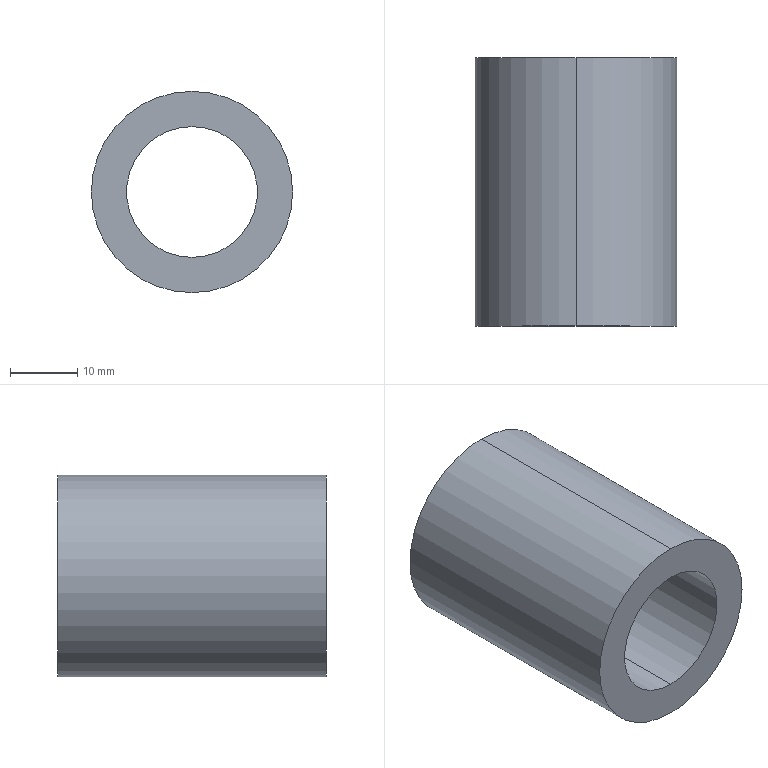Part | STEP file | 1 solid | 6 faces | box 30 x 40 x 30 mm | volume 16328 mm3 | cylinder 4 | plane 2 | commonest cylinder face diameters 19.5 x2 30 x2
STEP:
#1=CARTESIAN_POINT('',(0.,0.,0.));
#2=DIRECTION('',(0.,0.,1.));
#3=DIRECTION('',(1.,0.,0.));
#4=AXIS2_PLACEMENT_3D('',#1,#2,#3);
#5=CARTESIAN_POINT('',(0.,40.,-9.75));
#6=VERTEX_POINT('',#5);
#7=CARTESIAN_POINT('',(0.,0.,-9.75));
#8=VERTEX_POINT('',#7);
#9=CARTESIAN_POINT('',(0.,40.,-9.75));
#10=DIRECTION('',(0.,-1.,0.));
#11=VECTOR('',#10,1.);
#12=LINE('',#9,#11);
#13=CARTESIAN_POINT('',(0.,40.,0.));
#14=DIRECTION('',(0.,-1.,0.));
#15=DIRECTION('',(0.,0.,-1.));
#16=AXIS2_PLACEMENT_3D('',#13,#14,#15);
#17=CYLINDRICAL_SURFACE('',#16,9.75);
#18=CARTESIAN_POINT('',(6.283,0.));
#19=DIRECTION('',(0.,1.));
#20=VECTOR('',#19,1.);
#21=LINE('',#18,#20);
#22=(GEOMETRIC_REPRESENTATION_CONTEXT(2)PARAMETRIC_REPRESENTATION_CONTEXT()REPRESENTATION_CONTEXT('',''));
#23=DEFINITIONAL_REPRESENTATION('',(#21),#22);
#24=PCURVE('',#17,#23);
#25=CARTESIAN_POINT('',(0.,40.,0.));
#26=DIRECTION('',(0.,-1.,0.));
#27=DIRECTION('',(0.,0.,-1.));
#28=AXIS2_PLACEMENT_3D('',#25,#26,#27);
#29=CYLINDRICAL_SURFACE('',#28,9.75);
#30=CARTESIAN_POINT('',(0.,0.));
#31=DIRECTION('',(0.,1.));
#32=VECTOR('',#31,1.);
#33=LINE('',#30,#32);
#34=(GEOMETRIC_REPRESENTATION_CONTEXT(2)PARAMETRIC_REPRESENTATION_CONTEXT()REPRESENTATION_CONTEXT('',''));
#35=DEFINITIONAL_REPRESENTATION('',(#33),#34);
#36=PCURVE('',#29,#35);
#37=SURFACE_CURVE('',#12,(#24,#36),.PCURVE_S1.);
#38=EDGE_CURVE('',#6,#8,#37,.T.);
#39=ORIENTED_EDGE('',*,*,#38,.T.);
#40=CARTESIAN_POINT('',(0.,0.,9.75));
#41=VERTEX_POINT('',#40);
#42=CARTESIAN_POINT('',(0.,0.,0.));
#43=DIRECTION('',(0.,1.,0.));
#44=DIRECTION('',(0.,0.,1.));
#45=AXIS2_PLACEMENT_3D('',#42,#43,#44);
#46=CIRCLE('',#45,9.75);
#47=CARTESIAN_POINT('',(9.425,40.));
#48=DIRECTION('',(-1.,0.));
#49=VECTOR('',#48,1.);
#50=LINE('',#47,#49);
#51=(GEOMETRIC_REPRESENTATION_CONTEXT(2)PARAMETRIC_REPRESENTATION_CONTEXT()REPRESENTATION_CONTEXT('',''));
#52=DEFINITIONAL_REPRESENTATION('',(#50),#51);
#53=PCURVE('',#17,#52);
#54=CARTESIAN_POINT('',(0.,0.,0.));
#55=DIRECTION('',(0.,1.,0.));
#56=DIRECTION('',(0.,0.,1.));
#57=AXIS2_PLACEMENT_3D('',#54,#55,#56);
#58=PLANE('',#57);
#59=CARTESIAN_POINT('',(0.,0.));
#60=DIRECTION('',(1.,0.));
#61=AXIS2_PLACEMENT_2D('',#59,#60);
#62=CIRCLE('',#61,9.75);
#63=(GEOMETRIC_REPRESENTATION_CONTEXT(2)PARAMETRIC_REPRESENTATION_CONTEXT()REPRESENTATION_CONTEXT('',''));
#64=DEFINITIONAL_REPRESENTATION('',(#62),#63);
#65=PCURVE('',#58,#64);
#66=SURFACE_CURVE('',#46,(#53,#65),.PCURVE_S1.);
#67=EDGE_CURVE('',#8,#41,#66,.T.);
#68=ORIENTED_EDGE('',*,*,#67,.T.);
#69=CARTESIAN_POINT('',(0.,40.,9.75));
#70=VERTEX_POINT('',#69);
#71=CARTESIAN_POINT('',(0.,40.,9.75));
#72=DIRECTION('',(0.,-1.,0.));
#73=VECTOR('',#72,1.);
#74=LINE('',#71,#73);
#75=CARTESIAN_POINT('',(3.142,0.));
#76=DIRECTION('',(0.,1.));
#77=VECTOR('',#76,1.);
#78=LINE('',#75,#77);
#79=(GEOMETRIC_REPRESENTATION_CONTEXT(2)PARAMETRIC_REPRESENTATION_CONTEXT()REPRESENTATION_CONTEXT('',''));
#80=DEFINITIONAL_REPRESENTATION('',(#78),#79);
#81=PCURVE('',#17,#80);
#82=CARTESIAN_POINT('',(3.142,0.));
#83=DIRECTION('',(0.,1.));
#84=VECTOR('',#83,1.);
#85=LINE('',#82,#84);
#86=(GEOMETRIC_REPRESENTATION_CONTEXT(2)PARAMETRIC_REPRESENTATION_CONTEXT()REPRESENTATION_CONTEXT('',''));
#87=DEFINITIONAL_REPRESENTATION('',(#85),#86);
#88=PCURVE('',#29,#87);
#89=SURFACE_CURVE('',#74,(#81,#88),.PCURVE_S1.);
#90=EDGE_CURVE('',#70,#41,#89,.T.);
#91=ORIENTED_EDGE('',*,*,#90,.F.);
#92=CARTESIAN_POINT('',(0.,40.,0.));
#93=DIRECTION('',(0.,1.,0.));
#94=DIRECTION('',(0.,0.,1.));
#95=AXIS2_PLACEMENT_3D('',#92,#93,#94);
#96=CIRCLE('',#95,9.75);
#97=CARTESIAN_POINT('',(9.425,0.));
#98=DIRECTION('',(-1.,0.));
#99=VECTOR('',#98,1.);
#100=LINE('',#97,#99);
#101=(GEOMETRIC_REPRESENTATION_CONTEXT(2)PARAMETRIC_REPRESENTATION_CONTEXT()REPRESENTATION_CONTEXT('',''));
#102=DEFINITIONAL_REPRESENTATION('',(#100),#101);
#103=PCURVE('',#17,#102);
#104=CARTESIAN_POINT('',(0.,40.,0.));
#105=DIRECTION('',(0.,1.,0.));
#106=DIRECTION('',(0.,0.,1.));
#107=AXIS2_PLACEMENT_3D('',#104,#105,#106);
#108=PLANE('',#107);
#109=CARTESIAN_POINT('',(0.,0.));
#110=DIRECTION('',(1.,0.));
#111=AXIS2_PLACEMENT_2D('',#109,#110);
#112=CIRCLE('',#111,9.75);
#113=(GEOMETRIC_REPRESENTATION_CONTEXT(2)PARAMETRIC_REPRESENTATION_CONTEXT()REPRESENTATION_CONTEXT('',''));
#114=DEFINITIONAL_REPRESENTATION('',(#112),#113);
#115=PCURVE('',#108,#114);
#116=SURFACE_CURVE('',#96,(#103,#115),.PCURVE_S1.);
#117=EDGE_CURVE('',#6,#70,#116,.T.);
#118=ORIENTED_EDGE('',*,*,#117,.F.);
#119=EDGE_LOOP('',(#39,#68,#91,#118));
#120=FACE_BOUND('',#119,.F.);
#121=ADVANCED_FACE('',(#120),#17,.F.);
#122=CARTESIAN_POINT('',(0.,40.,15.));
#123=VERTEX_POINT('',#122);
#124=CARTESIAN_POINT('',(0.,40.,-15.));
#125=VERTEX_POINT('',#124);
#126=CARTESIAN_POINT('',(0.,40.,0.));
#127=DIRECTION('',(0.,1.,0.));
#128=DIRECTION('',(0.,0.,1.));
#129=AXIS2_PLACEMENT_3D('',#126,#127,#128);
#130=CIRCLE('',#129,15.);
#131=CARTESIAN_POINT('',(0.,40.,0.));
#132=DIRECTION('',(0.,-1.,0.));
#133=DIRECTION('',(0.,0.,-1.));
#134=AXIS2_PLACEMENT_3D('',#131,#132,#133);
#135=CYLINDRICAL_SURFACE('',#134,15.);
#136=CARTESIAN_POINT('',(3.142,0.));
#137=DIRECTION('',(-1.,0.));
#138=VECTOR('',#137,1.);
#139=LINE('',#136,#138);
#140=(GEOMETRIC_REPRESENTATION_CONTEXT(2)PARAMETRIC_REPRESENTATION_CONTEXT()REPRESENTATION_CONTEXT('',''));
#141=DEFINITIONAL_REPRESENTATION('',(#139),#140);
#142=PCURVE('',#135,#141);
#143=CARTESIAN_POINT('',(0.,0.));
#144=DIRECTION('',(1.,0.));
#145=AXIS2_PLACEMENT_2D('',#143,#144);
#146=CIRCLE('',#145,15.);
#147=(GEOMETRIC_REPRESENTATION_CONTEXT(2)PARAMETRIC_REPRESENTATION_CONTEXT()REPRESENTATION_CONTEXT('',''));
#148=DEFINITIONAL_REPRESENTATION('',(#146),#147);
#149=PCURVE('',#108,#148);
#150=SURFACE_CURVE('',#130,(#142,#149),.PCURVE_S1.);
#151=EDGE_CURVE('',#123,#125,#150,.T.);
#152=ORIENTED_EDGE('',*,*,#151,.F.);
#153=CARTESIAN_POINT('',(0.,0.,15.));
#154=VERTEX_POINT('',#153);
#155=CARTESIAN_POINT('',(0.,40.,15.));
#156=DIRECTION('',(0.,-1.,0.));
#157=VECTOR('',#156,1.);
#158=LINE('',#155,#157);
#159=CARTESIAN_POINT('',(3.142,0.));
#160=DIRECTION('',(0.,1.));
#161=VECTOR('',#160,1.);
#162=LINE('',#159,#161);
#163=(GEOMETRIC_REPRESENTATION_CONTEXT(2)PARAMETRIC_REPRESENTATION_CONTEXT()REPRESENTATION_CONTEXT('',''));
#164=DEFINITIONAL_REPRESENTATION('',(#162),#163);
#165=PCURVE('',#135,#164);
#166=CARTESIAN_POINT('',(0.,40.,0.));
#167=DIRECTION('',(0.,-1.,0.));
#168=DIRECTION('',(0.,0.,-1.));
#169=AXIS2_PLACEMENT_3D('',#166,#167,#168);
#170=CYLINDRICAL_SURFACE('',#169,15.);
#171=CARTESIAN_POINT('',(3.142,0.));
#172=DIRECTION('',(0.,1.));
#173=VECTOR('',#172,1.);
#174=LINE('',#171,#173);
#175=(GEOMETRIC_REPRESENTATION_CONTEXT(2)PARAMETRIC_REPRESENTATION_CONTEXT()REPRESENTATION_CONTEXT('',''));
#176=DEFINITIONAL_REPRESENTATION('',(#174),#175);
#177=PCURVE('',#170,#176);
#178=SURFACE_CURVE('',#158,(#165,#177),.PCURVE_S1.);
#179=EDGE_CURVE('',#123,#154,#178,.T.);
#180=ORIENTED_EDGE('',*,*,#179,.T.);
#181=CARTESIAN_POINT('',(0.,0.,-15.));
#182=VERTEX_POINT('',#181);
#183=CARTESIAN_POINT('',(0.,0.,0.));
#184=DIRECTION('',(0.,1.,0.));
#185=DIRECTION('',(0.,0.,1.));
#186=AXIS2_PLACEMENT_3D('',#183,#184,#185);
#187=CIRCLE('',#186,15.);
#188=CARTESIAN_POINT('',(3.142,40.));
#189=DIRECTION('',(-1.,0.));
#190=VECTOR('',#189,1.);
#191=LINE('',#188,#190);
#192=(GEOMETRIC_REPRESENTATION_CONTEXT(2)PARAMETRIC_REPRESENTATION_CONTEXT()REPRESENTATION_CONTEXT('',''));
#193=DEFINITIONAL_REPRESENTATION('',(#191),#192);
#194=PCURVE('',#135,#193);
#195=CARTESIAN_POINT('',(0.,0.));
#196=DIRECTION('',(1.,0.));
#197=AXIS2_PLACEMENT_2D('',#195,#196);
#198=CIRCLE('',#197,15.);
#199=(GEOMETRIC_REPRESENTATION_CONTEXT(2)PARAMETRIC_REPRESENTATION_CONTEXT()REPRESENTATION_CONTEXT('',''));
#200=DEFINITIONAL_REPRESENTATION('',(#198),#199);
#201=PCURVE('',#58,#200);
#202=SURFACE_CURVE('',#187,(#194,#201),.PCURVE_S1.);
#203=EDGE_CURVE('',#154,#182,#202,.T.);
#204=ORIENTED_EDGE('',*,*,#203,.T.);
#205=CARTESIAN_POINT('',(0.,40.,-15.));
#206=DIRECTION('',(0.,-1.,0.));
#207=VECTOR('',#206,1.);
#208=LINE('',#205,#207);
#209=CARTESIAN_POINT('',(0.,0.));
#210=DIRECTION('',(0.,1.));
#211=VECTOR('',#210,1.);
#212=LINE('',#209,#211);
#213=(GEOMETRIC_REPRESENTATION_CONTEXT(2)PARAMETRIC_REPRESENTATION_CONTEXT()REPRESENTATION_CONTEXT('',''));
#214=DEFINITIONAL_REPRESENTATION('',(#212),#213);
#215=PCURVE('',#135,#214);
#216=CARTESIAN_POINT('',(6.283,0.));
#217=DIRECTION('',(0.,1.));
#218=VECTOR('',#217,1.);
#219=LINE('',#216,#218);
#220=(GEOMETRIC_REPRESENTATION_CONTEXT(2)PARAMETRIC_REPRESENTATION_CONTEXT()REPRESENTATION_CONTEXT('',''));
#221=DEFINITIONAL_REPRESENTATION('',(#219),#220);
#222=PCURVE('',#170,#221);
#223=SURFACE_CURVE('',#208,(#215,#222),.PCURVE_S1.);
#224=EDGE_CURVE('',#125,#182,#223,.T.);
#225=ORIENTED_EDGE('',*,*,#224,.F.);
#226=EDGE_LOOP('',(#152,#180,#204,#225));
#227=FACE_BOUND('',#226,.T.);
#228=ADVANCED_FACE('',(#227),#135,.T.);
#229=CARTESIAN_POINT('',(0.,40.,0.));
#230=DIRECTION('',(0.,1.,0.));
#231=DIRECTION('',(0.,0.,1.));
#232=AXIS2_PLACEMENT_3D('',#229,#230,#231);
#233=CIRCLE('',#232,15.);
#234=CARTESIAN_POINT('',(0.,0.));
#235=DIRECTION('',(1.,0.));
#236=AXIS2_PLACEMENT_2D('',#234,#235);
#237=CIRCLE('',#236,15.);
#238=(GEOMETRIC_REPRESENTATION_CONTEXT(2)PARAMETRIC_REPRESENTATION_CONTEXT()REPRESENTATION_CONTEXT('',''));
#239=DEFINITIONAL_REPRESENTATION('',(#237),#238);
#240=PCURVE('',#108,#239);
#241=CARTESIAN_POINT('',(9.425,0.));
#242=DIRECTION('',(-1.,0.));
#243=VECTOR('',#242,1.);
#244=LINE('',#241,#243);
#245=(GEOMETRIC_REPRESENTATION_CONTEXT(2)PARAMETRIC_REPRESENTATION_CONTEXT()REPRESENTATION_CONTEXT('',''));
#246=DEFINITIONAL_REPRESENTATION('',(#244),#245);
#247=PCURVE('',#170,#246);
#248=SURFACE_CURVE('',#233,(#240,#247),.PCURVE_S1.);
#249=EDGE_CURVE('',#125,#123,#248,.T.);
#250=ORIENTED_EDGE('',*,*,#249,.T.);
#251=ORIENTED_EDGE('',*,*,#151,.T.);
#252=EDGE_LOOP('',(#250,#251));
#253=FACE_BOUND('',#252,.T.);
#254=ORIENTED_EDGE('',*,*,#117,.F.);
#255=CARTESIAN_POINT('',(0.,40.,0.));
#256=DIRECTION('',(0.,1.,0.));
#257=DIRECTION('',(0.,0.,1.));
#258=AXIS2_PLACEMENT_3D('',#255,#256,#257);
#259=CIRCLE('',#258,9.75);
#260=CARTESIAN_POINT('',(0.,0.));
#261=DIRECTION('',(1.,0.));
#262=AXIS2_PLACEMENT_2D('',#260,#261);
#263=CIRCLE('',#262,9.75);
#264=(GEOMETRIC_REPRESENTATION_CONTEXT(2)PARAMETRIC_REPRESENTATION_CONTEXT()REPRESENTATION_CONTEXT('',''));
#265=DEFINITIONAL_REPRESENTATION('',(#263),#264);
#266=PCURVE('',#108,#265);
#267=CARTESIAN_POINT('',(3.142,0.));
#268=DIRECTION('',(-1.,0.));
#269=VECTOR('',#268,1.);
#270=LINE('',#267,#269);
#271=(GEOMETRIC_REPRESENTATION_CONTEXT(2)PARAMETRIC_REPRESENTATION_CONTEXT()REPRESENTATION_CONTEXT('',''));
#272=DEFINITIONAL_REPRESENTATION('',(#270),#271);
#273=PCURVE('',#29,#272);
#274=SURFACE_CURVE('',#259,(#266,#273),.PCURVE_S1.);
#275=EDGE_CURVE('',#70,#6,#274,.T.);
#276=ORIENTED_EDGE('',*,*,#275,.F.);
#277=EDGE_LOOP('',(#254,#276));
#278=FACE_BOUND('',#277,.T.);
#279=ADVANCED_FACE('',(#253,#278),#108,.T.);
#280=CARTESIAN_POINT('',(0.,0.,0.));
#281=DIRECTION('',(0.,1.,0.));
#282=DIRECTION('',(0.,0.,1.));
#283=AXIS2_PLACEMENT_3D('',#280,#281,#282);
#284=CIRCLE('',#283,15.);
#285=CARTESIAN_POINT('',(0.,0.));
#286=DIRECTION('',(1.,0.));
#287=AXIS2_PLACEMENT_2D('',#285,#286);
#288=CIRCLE('',#287,15.);
#289=(GEOMETRIC_REPRESENTATION_CONTEXT(2)PARAMETRIC_REPRESENTATION_CONTEXT()REPRESENTATION_CONTEXT('',''));
#290=DEFINITIONAL_REPRESENTATION('',(#288),#289);
#291=PCURVE('',#58,#290);
#292=CARTESIAN_POINT('',(9.425,40.));
#293=DIRECTION('',(-1.,0.));
#294=VECTOR('',#293,1.);
#295=LINE('',#292,#294);
#296=(GEOMETRIC_REPRESENTATION_CONTEXT(2)PARAMETRIC_REPRESENTATION_CONTEXT()REPRESENTATION_CONTEXT('',''));
#297=DEFINITIONAL_REPRESENTATION('',(#295),#296);
#298=PCURVE('',#170,#297);
#299=SURFACE_CURVE('',#284,(#291,#298),.PCURVE_S1.);
#300=EDGE_CURVE('',#182,#154,#299,.T.);
#301=ORIENTED_EDGE('',*,*,#300,.F.);
#302=ORIENTED_EDGE('',*,*,#203,.F.);
#303=EDGE_LOOP('',(#301,#302));
#304=FACE_BOUND('',#303,.T.);
#305=ORIENTED_EDGE('',*,*,#67,.T.);
#306=CARTESIAN_POINT('',(0.,0.,0.));
#307=DIRECTION('',(0.,1.,0.));
#308=DIRECTION('',(0.,0.,1.));
#309=AXIS2_PLACEMENT_3D('',#306,#307,#308);
#310=CIRCLE('',#309,9.75);
#311=CARTESIAN_POINT('',(0.,0.));
#312=DIRECTION('',(1.,0.));
#313=AXIS2_PLACEMENT_2D('',#311,#312);
#314=CIRCLE('',#313,9.75);
#315=(GEOMETRIC_REPRESENTATION_CONTEXT(2)PARAMETRIC_REPRESENTATION_CONTEXT()REPRESENTATION_CONTEXT('',''));
#316=DEFINITIONAL_REPRESENTATION('',(#314),#315);
#317=PCURVE('',#58,#316);
#318=CARTESIAN_POINT('',(3.142,40.));
#319=DIRECTION('',(-1.,0.));
#320=VECTOR('',#319,1.);
#321=LINE('',#318,#320);
#322=(GEOMETRIC_REPRESENTATION_CONTEXT(2)PARAMETRIC_REPRESENTATION_CONTEXT()REPRESENTATION_CONTEXT('',''));
#323=DEFINITIONAL_REPRESENTATION('',(#321),#322);
#324=PCURVE('',#29,#323);
#325=SURFACE_CURVE('',#310,(#317,#324),.PCURVE_S1.);
#326=EDGE_CURVE('',#41,#8,#325,.T.);
#327=ORIENTED_EDGE('',*,*,#326,.T.);
#328=EDGE_LOOP('',(#305,#327));
#329=FACE_BOUND('',#328,.T.);
#330=ADVANCED_FACE('',(#304,#329),#58,.F.);
#331=ORIENTED_EDGE('',*,*,#179,.F.);
#332=ORIENTED_EDGE('',*,*,#249,.F.);
#333=ORIENTED_EDGE('',*,*,#224,.T.);
#334=ORIENTED_EDGE('',*,*,#300,.T.);
#335=EDGE_LOOP('',(#331,#332,#333,#334));
#336=FACE_BOUND('',#335,.T.);
#337=ADVANCED_FACE('',(#336),#170,.T.);
#338=ORIENTED_EDGE('',*,*,#326,.T.);
#339=ORIENTED_EDGE('',*,*,#38,.F.);
#340=ORIENTED_EDGE('',*,*,#275,.F.);
#341=ORIENTED_EDGE('',*,*,#90,.T.);
#342=EDGE_LOOP('',(#338,#339,#340,#341));
#343=FACE_BOUND('',#342,.F.);
#344=ADVANCED_FACE('',(#343),#29,.F.);
#345=CLOSED_SHELL('',(#121,#228,#279,#330,#337,#344));
#346=MANIFOLD_SOLID_BREP('',#345);
#347=(LENGTH_UNIT()NAMED_UNIT(*)SI_UNIT(.MILLI.,.METRE.));
#348=UNCERTAINTY_MEASURE_WITH_UNIT(LENGTH_MEASURE(0.0000001),#347,'','');
#349=(NAMED_UNIT(*)PLANE_ANGLE_UNIT()SI_UNIT($,.RADIAN.));
#350=(NAMED_UNIT(*)SI_UNIT($,.STERADIAN.)SOLID_ANGLE_UNIT());
#351=(GEOMETRIC_REPRESENTATION_CONTEXT(3)GLOBAL_UNCERTAINTY_ASSIGNED_CONTEXT((#348))GLOBAL_UNIT_ASSIGNED_CONTEXT((#347,#349,#350))REPRESENTATION_CONTEXT('',''));
#352=ADVANCED_BREP_SHAPE_REPRESENTATION('',(#4,#346),#351);